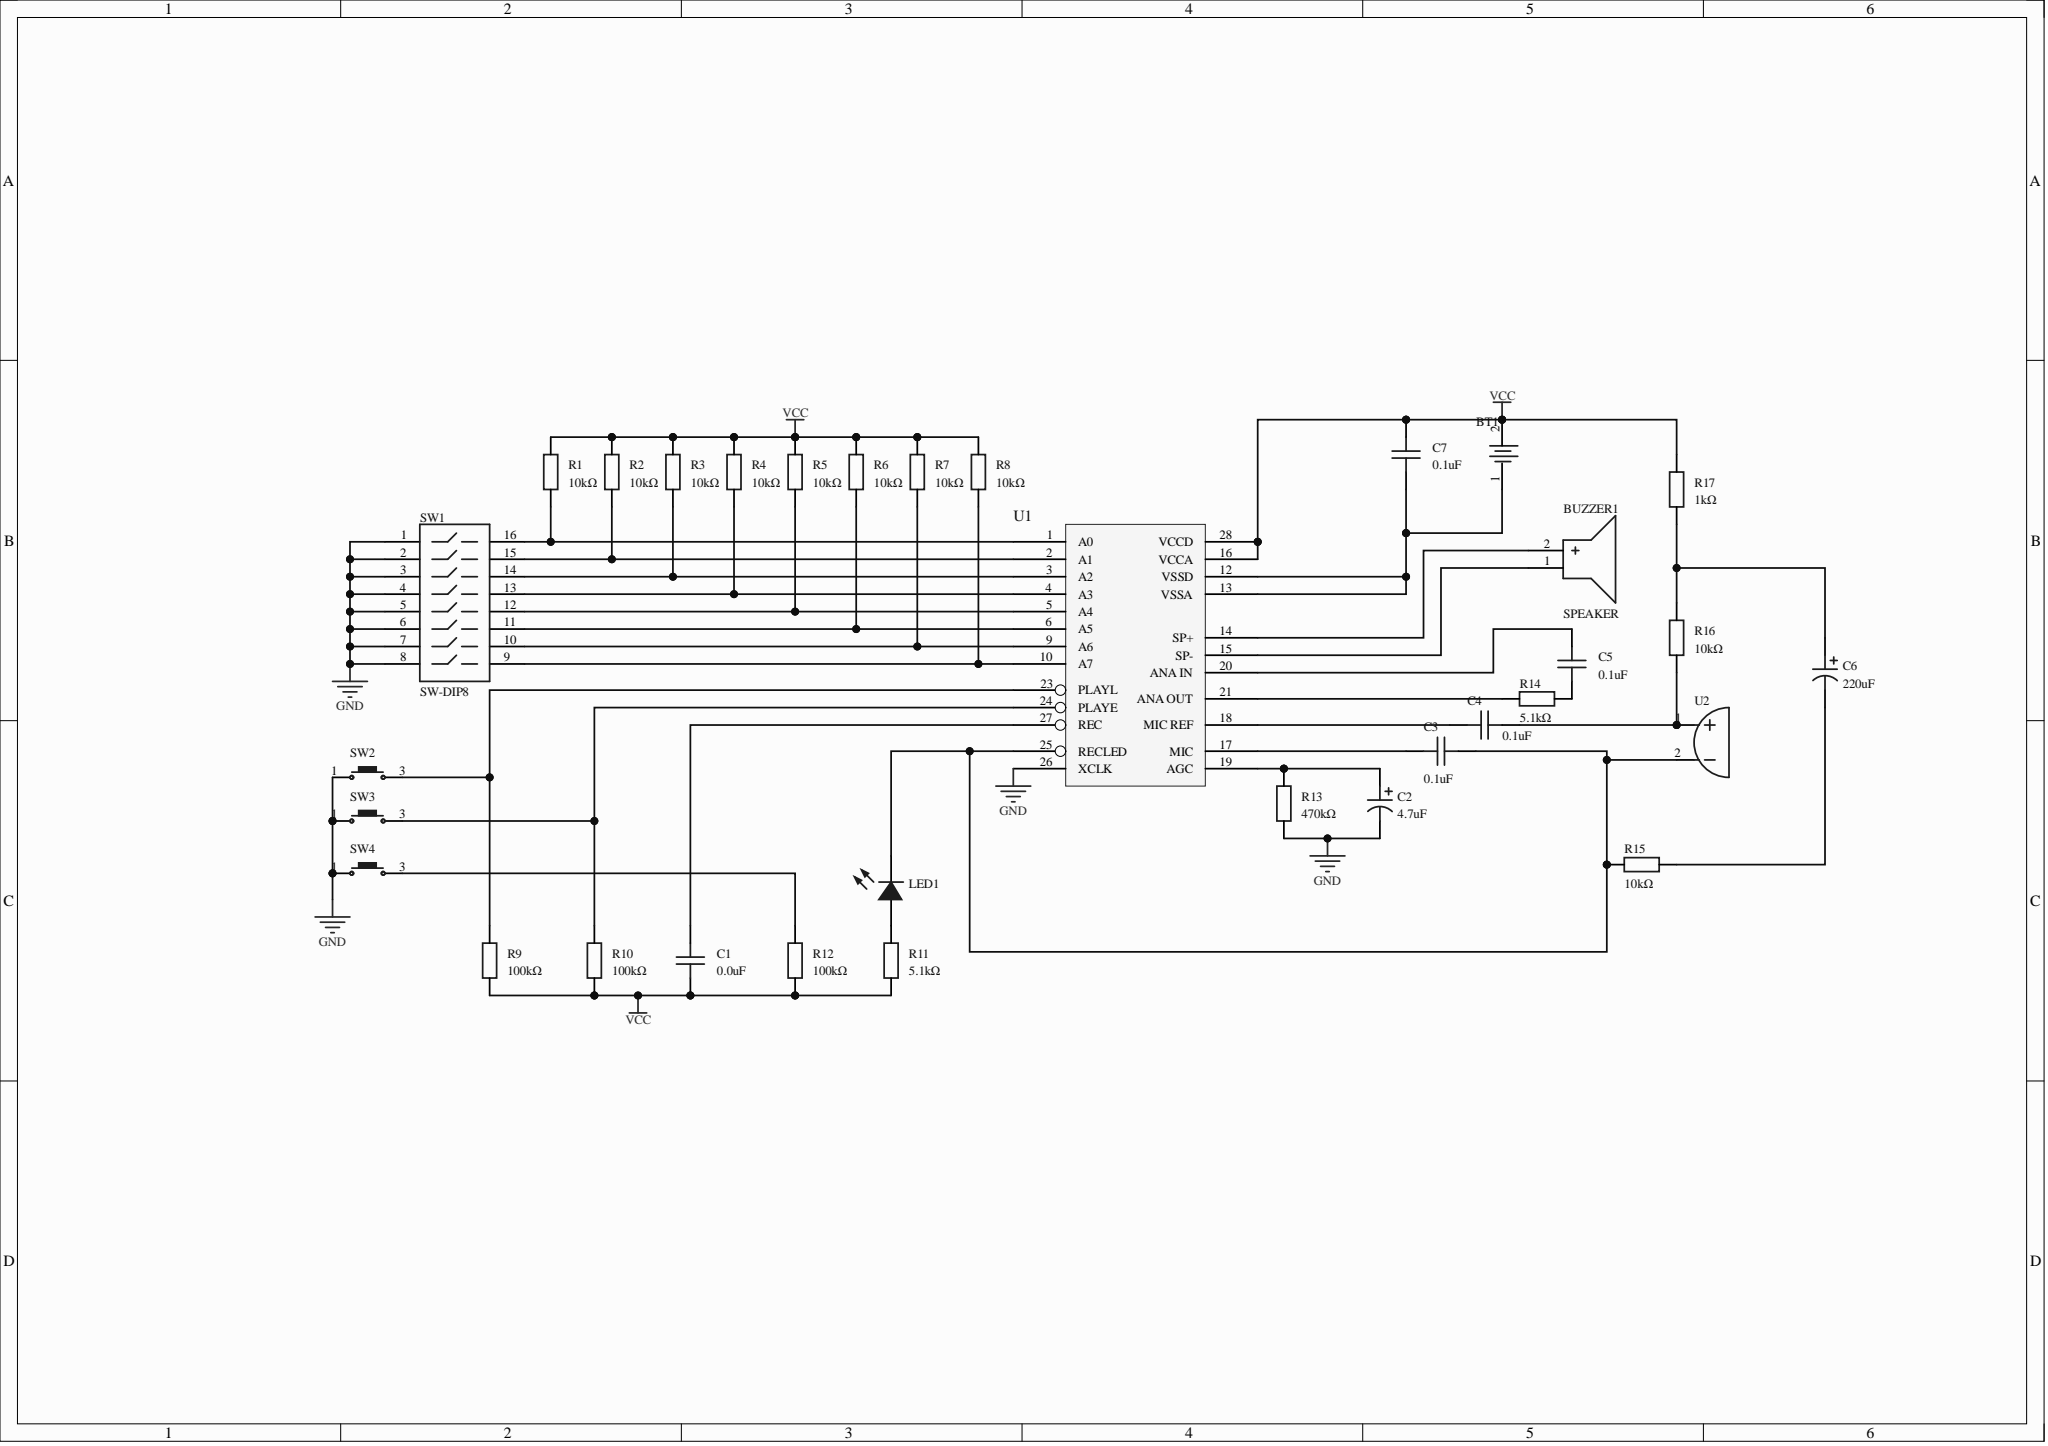Circuit board | Altium Designer | 33 parts | 28 nets
Bill of materials:
Comment,Description,Designator,Footprint,LibRef,Quantity
"","","BT1","HDR-TH_2P-P2.54-V-M-1","HDR-M_2.54_1x2P","1"
"SPEAKER","","BUZZER1","BUZ-TH_BD12.0-P6.00-D0.9-RD","buzzer","1"
"0.0uF","Capacitance:100nF;Tolerance:±10%;Rated voltage:50V;Temperature coefficient:X7R;","C1","CAP-TH_L5.1-W3.2-P5.08-D0.50","C323C104K5R5TA7301","1"
"4.7uF","Capacitance:10uF;Tolerance:±20%;Rated voltage:50V;Ripple current:120mA@100KHz;Equivalent series resistance(ESR):1.6Ω;","C2","CAP-TH_BD5.0-P2.00-D0.8-FD-10UF50VC110GL","10UF50VC110GL","1"
"0.1uF","Capacitance:100nF;Tolerance:±10%;Rated voltage:50V;Temperature coefficient:X7R;","C3, C4, C5, C7","CAP-TH_L5.1-W3.2-P5.08-D0.50","C323C104K5R5TA7301","4"
"220uF","Capacitance:10uF;Tolerance:±20%;Rated voltage:50V;Ripple current:120mA@100KHz;Equivalent series resistance(ESR):1.6Ω;","C6","CAP-TH_BD5.0-P2.00-D0.8-FD-10UF50VC110GL","10UF50VC110GL","1"
"","","LED1","LED_TH-3mm","LED_TH-B_3mm","1"
"10kΩ","","R1, R2, R3, R4, R5, R6, R7, R8, R15, R16","Res_1/4W","Res_AXIAL-1/4W","10"
"100kΩ","","R9, R10, R12","Res_1/8W","Res_AXIAL-1/8W","3"
"5.1kΩ","","R11","Res_1/8W","Res_AXIAL-1/8W","1"
"470kΩ","","R13","Res_1/4W","Res_AXIAL-1/4W","1"
"5.1kΩ","","R14","Res_1/4W","Res_AXIAL-1/4W","1"
"1kΩ","","R17","Res_1/4W","Res_AXIAL-1/4W","1"
"SW-DIP8","","SW1","SW-DIP8","SW-DIP8","1"
"","","SW2, SW3, SW4","SW-TH_4P-L6.0-W6.0-P4.50-LS6.5","Key_TH_6x6x6","3"
"","","U1, U2","","","2"
Netlist (Protel format):
[
BT1
HDR-TH_2P-P2.54-V-M-1




]
[
BUZZER1
BUZ-TH_BD12.0-P6.00-D0.9-RD
SPEAKER



]
[
C1
CAP-TH_L5.1-W3.2-P5.08-D0.50
0.0uF



]
[
C2
CAP-TH_BD5.0-P2.00-D0.8-FD-10UF50VC110GL
4.7uF



]
[
C3
CAP-TH_L5.1-W3.2-P5.08-D0.50
0.1uF



]
[
C4
CAP-TH_L5.1-W3.2-P5.08-D0.50
0.1uF



]
[
C5
CAP-TH_L5.1-W3.2-P5.08-D0.50
0.1uF



]
[
C6
CAP-TH_BD5.0-P2.00-D0.8-FD-10UF50VC110GL
220uF



]
[
C7
CAP-TH_L5.1-W3.2-P5.08-D0.50
0.1uF



]
[
LED1
LED_TH-3mm




]
[
R1
Res_1/4W
10kΩ



]
[
R2
Res_1/4W
10kΩ



]
[
R3
Res_1/4W
10kΩ



]
[
R4
Res_1/4W
10kΩ



]
[
R5
Res_1/4W
10kΩ



]
[
R6
Res_1/4W
10kΩ



]
[
R7
Res_1/4W
10kΩ



]
[
R8
Res_1/4W
10kΩ



]
[
R9
Res_1/8W
100kΩ



]
[
R10
Res_1/8W
100kΩ



]
[
R11
Res_1/8W
5.1kΩ



]
[
R12
Res_1/8W
100kΩ



]
[
R13
Res_1/4W
470kΩ



]
[
R14
Res_1/4W
5.1kΩ



]
[
R15
Res_1/4W
10kΩ



]
[
R16
Res_1/4W
10kΩ



]
[
R17
Res_1/4W
1kΩ



]
[
SW1
SW-DIP8
SW-DIP8



]
[
SW2
SW-TH_4P-L6.0-W6.0-P4.50-LS6.5




]
[
SW3
SW-TH_4P-L6.0-W6.0-P4.50-LS6.5




]
[
SW4
SW-TH_4P-L6.0-W6.0-P4.50-LS6.5




]
[
U1





]
[
U2





]
(
VCC
BT1-2
C1-1
C7-2
R1-2
R2-2
R3-2
R4-2
R5-2
R6-2
R7-2
R8-2
R9-1
R10-1
R11-1
R12-1
R17-2
U1-16
U1-28
)
(
NetR14_2
R14-2
U1-21
)
(
NetR12_2
R12-2
SW4-3
)
(
NetR10_2
R10-2
SW3-3
U1-24
)
(
NetR9_2
R9-2
SW2-3
U1-23
)
(
NetR8_1
R8-1
SW1-9
U1-10
)
(
NetR7_1
R7-1
SW1-10
U1-9
)
(
NetR6_1
R6-1
SW1-11
U1-6
)
(
NetR5_1
R5-1
SW1-12
U1-5
)
(
NetR4_1
R4-1
SW1-13
U1-4
)
(
NetR3_1
R3-1
SW1-14
U1-3
)
(
NetR2_1
R2-1
SW1-15
U1-2
)
(
NetR1_1
R1-1
SW1-16
U1-1
)
(
NetLED1_1
LED1-1
R11-2
)
(
NetC6_2
C6-2
R15-2
)
(
NetC6_1
C6-1
R16-2
R17-1
)
(
NetC5_2
C5-2
U1-20
)
(
NetC5_1
C5-1
R14-1
)
(
NetC4_2
C4-2
R16-1
U2-1
)
(
NetC4_1
C4-1
U1-18
)
(
NetC3_2
C3-2
LED1-2
R15-1
U1-25
U2-2
)
(
NetC3_1
C3-1
U1-17
)
(
NetC2_1
C2-1
R13-2
U1-19
)
(
NetC1_2
C1-2
U1-27
)
(
NetBUZZER1_2
BUZZER1-2
U1-14
)
(
NetBUZZER1_1
BUZZER1-1
U1-15
)
(
NetBT1_1
BT1-1
C7-1
U1-12
U1-13
)
(
GND
C2-2
R13-1
SW1-1
SW1-2
SW1-3
SW1-4
SW1-5
SW1-6
SW1-7
SW1-8
SW2-1
SW3-1
SW4-1
U1-26
)